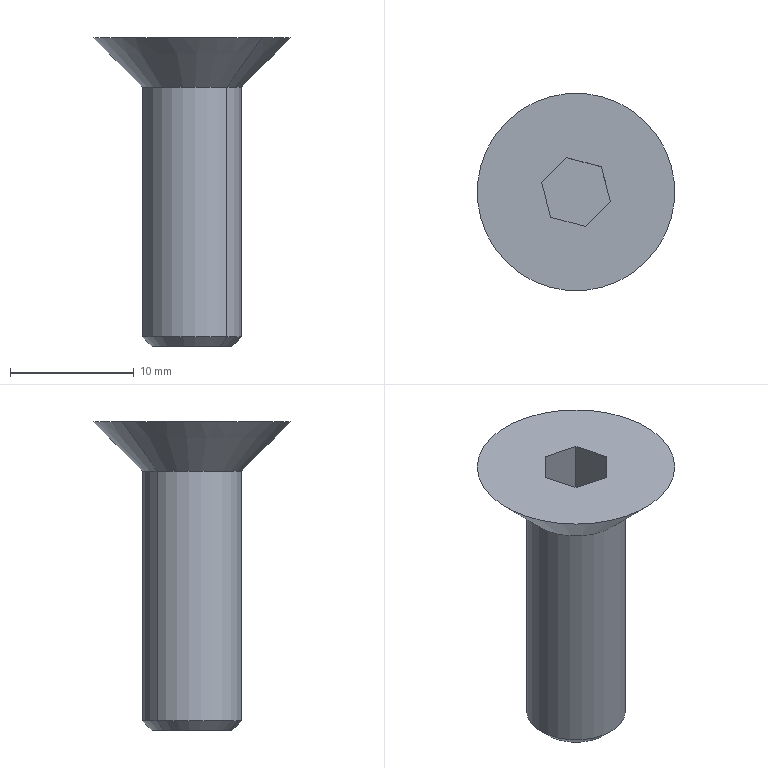Part | NX | features 2 2 | 1 solid | 15 faces | box 16 x 16 x 25 mm | volume 1423 mm3 | plane 9 | cone 4 | cylinder 2 | commonest cylinder face diameters 8 x2
STEP:
#1=CARTESIAN_POINT('',(149.328,-302.828,127.667));
#2=VERTEX_POINT('',#1);
#3=CARTESIAN_POINT('',(148.786,-302.286,126.9));
#4=VERTEX_POINT('',#3);
#5=CARTESIAN_POINT('',(149.057,-302.557,127.284));
#6=DIRECTION('',(-0.5,0.5,-0.7071));
#7=VECTOR('',#6,1000.);
#8=LINE('',#5,#7);
#9=EDGE_CURVE('',#2,#4,#8,.T.);
#10=ORIENTED_EDGE('',*,*,#9,.F.);
#11=CARTESIAN_POINT('',(143.672,-297.172,127.667));
#12=VERTEX_POINT('',#11);
#13=CARTESIAN_POINT('',(146.5,-300.,127.667));
#14=DIRECTION('',(0.,0.,-1.));
#15=DIRECTION('',(0.7071,-0.7071,0.));
#16=AXIS2_PLACEMENT_3D('',#13,#14,#15);
#17=CIRCLE('',#16,4.);
#18=EDGE_CURVE('',#2,#12,#17,.T.);
#19=ORIENTED_EDGE('',*,*,#18,.T.);
#20=CARTESIAN_POINT('',(144.214,-297.714,126.9));
#21=VERTEX_POINT('',#20);
#22=CARTESIAN_POINT('',(143.943,-297.443,127.284));
#23=DIRECTION('',(-0.5,0.5,0.7071));
#24=VECTOR('',#23,1000.);
#25=LINE('',#22,#24);
#26=EDGE_CURVE('',#21,#12,#25,.T.);
#27=ORIENTED_EDGE('',*,*,#26,.F.);
#28=CARTESIAN_POINT('',(146.5,-300.,126.9));
#29=DIRECTION('',(0.,0.,-1.));
#30=DIRECTION('',(0.7071,-0.7071,0.));
#31=AXIS2_PLACEMENT_3D('',#28,#29,#30);
#32=CIRCLE('',#31,3.233);
#33=EDGE_CURVE('',#4,#21,#32,.T.);
#34=ORIENTED_EDGE('',*,*,#33,.F.);
#35=EDGE_LOOP('',(#10,#19,#27,#34));
#36=FACE_BOUND('',#35,.T.);
#37=CARTESIAN_POINT('',(146.5,-300.,127.284));
#38=DIRECTION('',(0.,0.,1.));
#39=DIRECTION('',(0.7071,-0.7071,0.));
#40=AXIS2_PLACEMENT_3D('',#37,#38,#39);
#41=CONICAL_SURFACE('',#40,3.616,0.7854);
#42=ADVANCED_FACE('',(#36),#41,.T.);
#43=CARTESIAN_POINT('',(149.328,-302.828,147.9));
#44=VERTEX_POINT('',#43);
#45=CARTESIAN_POINT('',(149.328,-302.828,137.784));
#46=DIRECTION('',(0.,0.,-1.));
#47=VECTOR('',#46,1000.);
#48=LINE('',#45,#47);
#49=EDGE_CURVE('',#44,#2,#48,.T.);
#50=ORIENTED_EDGE('',*,*,#49,.F.);
#51=CARTESIAN_POINT('',(143.672,-297.172,147.9));
#52=VERTEX_POINT('',#51);
#53=CARTESIAN_POINT('',(146.5,-300.,147.9));
#54=DIRECTION('',(0.,0.,-1.));
#55=DIRECTION('',(0.7071,-0.7071,0.));
#56=AXIS2_PLACEMENT_3D('',#53,#54,#55);
#57=CIRCLE('',#56,4.);
#58=EDGE_CURVE('',#44,#52,#57,.T.);
#59=ORIENTED_EDGE('',*,*,#58,.T.);
#60=CARTESIAN_POINT('',(143.672,-297.172,137.784));
#61=DIRECTION('',(0.,0.,1.));
#62=VECTOR('',#61,1000.);
#63=LINE('',#60,#62);
#64=EDGE_CURVE('',#12,#52,#63,.T.);
#65=ORIENTED_EDGE('',*,*,#64,.F.);
#66=ORIENTED_EDGE('',*,*,#18,.F.);
#67=EDGE_LOOP('',(#50,#59,#65,#66));
#68=FACE_BOUND('',#67,.T.);
#69=CARTESIAN_POINT('',(146.5,-300.,137.784));
#70=DIRECTION('',(0.,0.,1.));
#71=DIRECTION('',(0.7071,-0.7071,0.));
#72=AXIS2_PLACEMENT_3D('',#69,#70,#71);
#73=CYLINDRICAL_SURFACE('',#72,4.);
#74=ADVANCED_FACE('',(#68),#73,.T.);
#75=CARTESIAN_POINT('',(152.157,-305.657,151.9));
#76=VERTEX_POINT('',#75);
#77=CARTESIAN_POINT('',(150.743,-304.243,149.9));
#78=DIRECTION('',(-0.5,0.5,-0.7071));
#79=VECTOR('',#78,1000.);
#80=LINE('',#77,#79);
#81=EDGE_CURVE('',#76,#44,#80,.T.);
#82=ORIENTED_EDGE('',*,*,#81,.F.);
#83=CARTESIAN_POINT('',(140.843,-294.343,151.9));
#84=VERTEX_POINT('',#83);
#85=CARTESIAN_POINT('',(146.5,-300.,151.9));
#86=DIRECTION('',(0.,0.,-1.));
#87=DIRECTION('',(0.7071,-0.7071,0.));
#88=AXIS2_PLACEMENT_3D('',#85,#86,#87);
#89=CIRCLE('',#88,8.);
#90=EDGE_CURVE('',#76,#84,#89,.T.);
#91=ORIENTED_EDGE('',*,*,#90,.T.);
#92=CARTESIAN_POINT('',(142.257,-295.757,149.9));
#93=DIRECTION('',(-0.5,0.5,0.7071));
#94=VECTOR('',#93,1000.);
#95=LINE('',#92,#94);
#96=EDGE_CURVE('',#52,#84,#95,.T.);
#97=ORIENTED_EDGE('',*,*,#96,.F.);
#98=ORIENTED_EDGE('',*,*,#58,.F.);
#99=EDGE_LOOP('',(#82,#91,#97,#98));
#100=FACE_BOUND('',#99,.T.);
#101=CARTESIAN_POINT('',(146.5,-300.,149.9));
#102=DIRECTION('',(0.,0.,1.));
#103=DIRECTION('',(0.7071,-0.7071,0.));
#104=AXIS2_PLACEMENT_3D('',#101,#102,#103);
#105=CONICAL_SURFACE('',#104,6.,0.7854);
#106=ADVANCED_FACE('',(#100),#105,.T.);
#107=CARTESIAN_POINT('',(143.712,-299.253,147.5));
#108=VERTEX_POINT('',#107);
#109=CARTESIAN_POINT('',(144.459,-302.041,147.5));
#110=VERTEX_POINT('',#109);
#111=CARTESIAN_POINT('',(143.712,-299.253,147.5));
#112=DIRECTION('',(0.2588,-0.9659,0.));
#113=VECTOR('',#112,1000.);
#114=LINE('',#111,#113);
#115=EDGE_CURVE('',#108,#110,#114,.T.);
#116=ORIENTED_EDGE('',*,*,#115,.F.);
#117=CARTESIAN_POINT('',(143.712,-299.253,151.9));
#118=VERTEX_POINT('',#117);
#119=CARTESIAN_POINT('',(143.712,-299.253,151.9));
#120=DIRECTION('',(0.,0.,-1.));
#121=VECTOR('',#120,1000.);
#122=LINE('',#119,#121);
#123=EDGE_CURVE('',#118,#108,#122,.T.);
#124=ORIENTED_EDGE('',*,*,#123,.F.);
#125=CARTESIAN_POINT('',(144.459,-302.041,151.9));
#126=VERTEX_POINT('',#125);
#127=CARTESIAN_POINT('',(144.347,-301.623,151.9));
#128=DIRECTION('',(-0.2588,0.9659,0.));
#129=VECTOR('',#128,1000.);
#130=LINE('',#127,#129);
#131=EDGE_CURVE('',#126,#118,#130,.T.);
#132=ORIENTED_EDGE('',*,*,#131,.F.);
#133=CARTESIAN_POINT('',(144.459,-302.041,151.9));
#134=DIRECTION('',(0.,0.,-1.));
#135=VECTOR('',#134,1000.);
#136=LINE('',#133,#135);
#137=EDGE_CURVE('',#126,#110,#136,.T.);
#138=ORIENTED_EDGE('',*,*,#137,.T.);
#139=EDGE_LOOP('',(#116,#124,#132,#138));
#140=FACE_BOUND('',#139,.T.);
#141=CARTESIAN_POINT('',(143.712,-299.253,151.9));
#142=DIRECTION('',(-0.9659,-0.2588,0.));
#143=DIRECTION('',(-0.2588,0.9659,0.));
#144=AXIS2_PLACEMENT_3D('',#141,#142,#143);
#145=PLANE('',#144);
#146=ADVANCED_FACE('',(#140),#145,.F.);
#147=CARTESIAN_POINT('',(147.247,-302.788,147.5));
#148=VERTEX_POINT('',#147);
#149=CARTESIAN_POINT('',(144.459,-302.041,147.5));
#150=DIRECTION('',(0.9659,-0.2588,0.));
#151=VECTOR('',#150,1000.);
#152=LINE('',#149,#151);
#153=EDGE_CURVE('',#110,#148,#152,.T.);
#154=ORIENTED_EDGE('',*,*,#153,.F.);
#155=ORIENTED_EDGE('',*,*,#137,.F.);
#156=CARTESIAN_POINT('',(147.247,-302.788,151.9));
#157=VERTEX_POINT('',#156);
#158=CARTESIAN_POINT('',(146.829,-302.676,151.9));
#159=DIRECTION('',(-0.9659,0.2588,0.));
#160=VECTOR('',#159,1000.);
#161=LINE('',#158,#160);
#162=EDGE_CURVE('',#157,#126,#161,.T.);
#163=ORIENTED_EDGE('',*,*,#162,.F.);
#164=CARTESIAN_POINT('',(147.247,-302.788,151.9));
#165=DIRECTION('',(0.,0.,-1.));
#166=VECTOR('',#165,1000.);
#167=LINE('',#164,#166);
#168=EDGE_CURVE('',#157,#148,#167,.T.);
#169=ORIENTED_EDGE('',*,*,#168,.T.);
#170=EDGE_LOOP('',(#154,#155,#163,#169));
#171=FACE_BOUND('',#170,.T.);
#172=CARTESIAN_POINT('',(144.459,-302.041,151.9));
#173=DIRECTION('',(-0.2588,-0.9659,0.));
#174=DIRECTION('',(-0.9659,0.2588,0.));
#175=AXIS2_PLACEMENT_3D('',#172,#173,#174);
#176=PLANE('',#175);
#177=ADVANCED_FACE('',(#171),#176,.F.);
#178=CARTESIAN_POINT('',(149.288,-300.747,147.5));
#179=VERTEX_POINT('',#178);
#180=CARTESIAN_POINT('',(147.247,-302.788,147.5));
#181=DIRECTION('',(0.7071,0.7071,0.));
#182=VECTOR('',#181,1000.);
#183=LINE('',#180,#182);
#184=EDGE_CURVE('',#148,#179,#183,.T.);
#185=ORIENTED_EDGE('',*,*,#184,.F.);
#186=ORIENTED_EDGE('',*,*,#168,.F.);
#187=CARTESIAN_POINT('',(149.288,-300.747,151.9));
#188=VERTEX_POINT('',#187);
#189=CARTESIAN_POINT('',(147.757,-302.278,151.9));
#190=DIRECTION('',(-0.7071,-0.7071,0.));
#191=VECTOR('',#190,1000.);
#192=LINE('',#189,#191);
#193=EDGE_CURVE('',#188,#157,#192,.T.);
#194=ORIENTED_EDGE('',*,*,#193,.F.);
#195=CARTESIAN_POINT('',(149.288,-300.747,151.9));
#196=DIRECTION('',(0.,0.,-1.));
#197=VECTOR('',#196,1000.);
#198=LINE('',#195,#197);
#199=EDGE_CURVE('',#188,#179,#198,.T.);
#200=ORIENTED_EDGE('',*,*,#199,.T.);
#201=EDGE_LOOP('',(#185,#186,#194,#200));
#202=FACE_BOUND('',#201,.T.);
#203=CARTESIAN_POINT('',(147.247,-302.788,151.9));
#204=DIRECTION('',(0.7071,-0.7071,0.));
#205=DIRECTION('',(-0.7071,-0.7071,0.));
#206=AXIS2_PLACEMENT_3D('',#203,#204,#205);
#207=PLANE('',#206);
#208=ADVANCED_FACE('',(#202),#207,.F.);
#209=CARTESIAN_POINT('',(148.541,-297.959,147.5));
#210=VERTEX_POINT('',#209);
#211=CARTESIAN_POINT('',(149.288,-300.747,147.5));
#212=DIRECTION('',(-0.2588,0.9659,0.));
#213=VECTOR('',#212,1000.);
#214=LINE('',#211,#213);
#215=EDGE_CURVE('',#179,#210,#214,.T.);
#216=ORIENTED_EDGE('',*,*,#215,.F.);
#217=ORIENTED_EDGE('',*,*,#199,.F.);
#218=CARTESIAN_POINT('',(148.541,-297.959,151.9));
#219=VERTEX_POINT('',#218);
#220=CARTESIAN_POINT('',(149.55,-301.723,151.9));
#221=DIRECTION('',(0.2588,-0.9659,0.));
#222=VECTOR('',#221,1000.);
#223=LINE('',#220,#222);
#224=EDGE_CURVE('',#219,#188,#223,.T.);
#225=ORIENTED_EDGE('',*,*,#224,.F.);
#226=CARTESIAN_POINT('',(148.541,-297.959,151.9));
#227=DIRECTION('',(0.,0.,-1.));
#228=VECTOR('',#227,1000.);
#229=LINE('',#226,#228);
#230=EDGE_CURVE('',#219,#210,#229,.T.);
#231=ORIENTED_EDGE('',*,*,#230,.T.);
#232=EDGE_LOOP('',(#216,#217,#225,#231));
#233=FACE_BOUND('',#232,.T.);
#234=CARTESIAN_POINT('',(149.288,-300.747,151.9));
#235=DIRECTION('',(0.9659,0.2588,0.));
#236=DIRECTION('',(0.2588,-0.9659,0.));
#237=AXIS2_PLACEMENT_3D('',#234,#235,#236);
#238=PLANE('',#237);
#239=ADVANCED_FACE('',(#233),#238,.F.);
#240=CARTESIAN_POINT('',(145.753,-297.212,147.5));
#241=VERTEX_POINT('',#240);
#242=CARTESIAN_POINT('',(148.541,-297.959,147.5));
#243=DIRECTION('',(-0.9659,0.2588,0.));
#244=VECTOR('',#243,1000.);
#245=LINE('',#242,#244);
#246=EDGE_CURVE('',#210,#241,#245,.T.);
#247=ORIENTED_EDGE('',*,*,#246,.F.);
#248=ORIENTED_EDGE('',*,*,#230,.F.);
#249=CARTESIAN_POINT('',(145.753,-297.212,151.9));
#250=VERTEX_POINT('',#249);
#251=CARTESIAN_POINT('',(149.517,-298.22,151.9));
#252=DIRECTION('',(0.9659,-0.2588,0.));
#253=VECTOR('',#252,1000.);
#254=LINE('',#251,#253);
#255=EDGE_CURVE('',#250,#219,#254,.T.);
#256=ORIENTED_EDGE('',*,*,#255,.F.);
#257=CARTESIAN_POINT('',(145.753,-297.212,151.9));
#258=DIRECTION('',(0.,0.,-1.));
#259=VECTOR('',#258,1000.);
#260=LINE('',#257,#259);
#261=EDGE_CURVE('',#250,#241,#260,.T.);
#262=ORIENTED_EDGE('',*,*,#261,.T.);
#263=EDGE_LOOP('',(#247,#248,#256,#262));
#264=FACE_BOUND('',#263,.T.);
#265=CARTESIAN_POINT('',(148.541,-297.959,151.9));
#266=DIRECTION('',(0.2588,0.9659,0.));
#267=DIRECTION('',(0.9659,-0.2588,0.));
#268=AXIS2_PLACEMENT_3D('',#265,#266,#267);
#269=PLANE('',#268);
#270=ADVANCED_FACE('',(#264),#269,.F.);
#271=CARTESIAN_POINT('',(145.753,-297.212,147.5));
#272=DIRECTION('',(-0.7071,-0.7071,0.));
#273=VECTOR('',#272,1000.);
#274=LINE('',#271,#273);
#275=EDGE_CURVE('',#241,#108,#274,.T.);
#276=ORIENTED_EDGE('',*,*,#275,.F.);
#277=ORIENTED_EDGE('',*,*,#261,.F.);
#278=CARTESIAN_POINT('',(145.243,-297.722,151.9));
#279=DIRECTION('',(0.7071,0.7071,0.));
#280=VECTOR('',#279,1000.);
#281=LINE('',#278,#280);
#282=EDGE_CURVE('',#118,#250,#281,.T.);
#283=ORIENTED_EDGE('',*,*,#282,.F.);
#284=ORIENTED_EDGE('',*,*,#123,.T.);
#285=EDGE_LOOP('',(#276,#277,#283,#284));
#286=FACE_BOUND('',#285,.T.);
#287=CARTESIAN_POINT('',(145.753,-297.212,151.9));
#288=DIRECTION('',(-0.7071,0.7071,0.));
#289=DIRECTION('',(0.7071,0.7071,0.));
#290=AXIS2_PLACEMENT_3D('',#287,#288,#289);
#291=PLANE('',#290);
#292=ADVANCED_FACE('',(#286),#291,.F.);
#293=ORIENTED_EDGE('',*,*,#115,.T.);
#294=ORIENTED_EDGE('',*,*,#153,.T.);
#295=ORIENTED_EDGE('',*,*,#184,.T.);
#296=ORIENTED_EDGE('',*,*,#215,.T.);
#297=ORIENTED_EDGE('',*,*,#246,.T.);
#298=ORIENTED_EDGE('',*,*,#275,.T.);
#299=EDGE_LOOP('',(#293,#294,#295,#296,#297,#298));
#300=FACE_BOUND('',#299,.T.);
#301=CARTESIAN_POINT('',(146.5,-300.,147.5));
#302=DIRECTION('',(0.,0.,1.));
#303=DIRECTION('',(0.7071,-0.7071,0.));
#304=AXIS2_PLACEMENT_3D('',#301,#302,#303);
#305=PLANE('',#304);
#306=ADVANCED_FACE('',(#300),#305,.T.);
#307=ORIENTED_EDGE('',*,*,#131,.T.);
#308=ORIENTED_EDGE('',*,*,#282,.T.);
#309=ORIENTED_EDGE('',*,*,#255,.T.);
#310=ORIENTED_EDGE('',*,*,#224,.T.);
#311=ORIENTED_EDGE('',*,*,#193,.T.);
#312=ORIENTED_EDGE('',*,*,#162,.T.);
#313=EDGE_LOOP('',(#307,#308,#309,#310,#311,#312));
#314=FACE_BOUND('',#313,.T.);
#315=ORIENTED_EDGE('',*,*,#90,.F.);
#316=CARTESIAN_POINT('',(146.5,-300.,151.9));
#317=DIRECTION('',(0.,0.,-1.));
#318=DIRECTION('',(0.7071,-0.7071,0.));
#319=AXIS2_PLACEMENT_3D('',#316,#317,#318);
#320=CIRCLE('',#319,8.);
#321=EDGE_CURVE('',#84,#76,#320,.T.);
#322=ORIENTED_EDGE('',*,*,#321,.F.);
#323=EDGE_LOOP('',(#315,#322));
#324=FACE_BOUND('',#323,.T.);
#325=CARTESIAN_POINT('',(149.328,-302.828,151.9));
#326=DIRECTION('',(0.,0.,1.));
#327=DIRECTION('',(-0.7071,0.7071,0.));
#328=AXIS2_PLACEMENT_3D('',#325,#326,#327);
#329=PLANE('',#328);
#330=ADVANCED_FACE('',(#314,#324),#329,.T.);
#331=ORIENTED_EDGE('',*,*,#81,.T.);
#332=CARTESIAN_POINT('',(146.5,-300.,147.9));
#333=DIRECTION('',(0.,0.,-1.));
#334=DIRECTION('',(0.7071,-0.7071,0.));
#335=AXIS2_PLACEMENT_3D('',#332,#333,#334);
#336=CIRCLE('',#335,4.);
#337=EDGE_CURVE('',#52,#44,#336,.T.);
#338=ORIENTED_EDGE('',*,*,#337,.F.);
#339=ORIENTED_EDGE('',*,*,#96,.T.);
#340=ORIENTED_EDGE('',*,*,#321,.T.);
#341=EDGE_LOOP('',(#331,#338,#339,#340));
#342=FACE_BOUND('',#341,.T.);
#343=CARTESIAN_POINT('',(146.5,-300.,149.9));
#344=DIRECTION('',(0.,0.,1.));
#345=DIRECTION('',(0.7071,-0.7071,0.));
#346=AXIS2_PLACEMENT_3D('',#343,#344,#345);
#347=CONICAL_SURFACE('',#346,6.,0.7854);
#348=ADVANCED_FACE('',(#342),#347,.T.);
#349=ORIENTED_EDGE('',*,*,#49,.T.);
#350=CARTESIAN_POINT('',(146.5,-300.,127.667));
#351=DIRECTION('',(0.,0.,-1.));
#352=DIRECTION('',(0.7071,-0.7071,0.));
#353=AXIS2_PLACEMENT_3D('',#350,#351,#352);
#354=CIRCLE('',#353,4.);
#355=EDGE_CURVE('',#12,#2,#354,.T.);
#356=ORIENTED_EDGE('',*,*,#355,.F.);
#357=ORIENTED_EDGE('',*,*,#64,.T.);
#358=ORIENTED_EDGE('',*,*,#337,.T.);
#359=EDGE_LOOP('',(#349,#356,#357,#358));
#360=FACE_BOUND('',#359,.T.);
#361=CARTESIAN_POINT('',(146.5,-300.,137.784));
#362=DIRECTION('',(0.,0.,1.));
#363=DIRECTION('',(0.7071,-0.7071,0.));
#364=AXIS2_PLACEMENT_3D('',#361,#362,#363);
#365=CYLINDRICAL_SURFACE('',#364,4.);
#366=ADVANCED_FACE('',(#360),#365,.T.);
#367=ORIENTED_EDGE('',*,*,#9,.T.);
#368=CARTESIAN_POINT('',(146.5,-300.,126.9));
#369=DIRECTION('',(0.,0.,-1.));
#370=DIRECTION('',(0.7071,-0.7071,0.));
#371=AXIS2_PLACEMENT_3D('',#368,#369,#370);
#372=CIRCLE('',#371,3.233);
#373=EDGE_CURVE('',#21,#4,#372,.T.);
#374=ORIENTED_EDGE('',*,*,#373,.F.);
#375=ORIENTED_EDGE('',*,*,#26,.T.);
#376=ORIENTED_EDGE('',*,*,#355,.T.);
#377=EDGE_LOOP('',(#367,#374,#375,#376));
#378=FACE_BOUND('',#377,.T.);
#379=CARTESIAN_POINT('',(146.5,-300.,127.284));
#380=DIRECTION('',(0.,0.,1.));
#381=DIRECTION('',(0.7071,-0.7071,0.));
#382=AXIS2_PLACEMENT_3D('',#379,#380,#381);
#383=CONICAL_SURFACE('',#382,3.616,0.7854);
#384=ADVANCED_FACE('',(#378),#383,.T.);
#385=ORIENTED_EDGE('',*,*,#33,.T.);
#386=ORIENTED_EDGE('',*,*,#373,.T.);
#387=EDGE_LOOP('',(#385,#386));
#388=FACE_BOUND('',#387,.T.);
#389=CARTESIAN_POINT('',(147.643,-301.143,126.9));
#390=DIRECTION('',(0.,0.,-1.));
#391=DIRECTION('',(0.7071,-0.7071,0.));
#392=AXIS2_PLACEMENT_3D('',#389,#390,#391);
#393=PLANE('',#392);
#394=ADVANCED_FACE('',(#388),#393,.T.);
#395=CLOSED_SHELL('',(#42,#74,#106,#146,#177,#208,#239,#270,#292,#306,#330,#348,#366,#384,#394));
#396=MANIFOLD_SOLID_BREP('',#395);
#397=(LENGTH_UNIT()NAMED_UNIT(*)SI_UNIT(.MILLI.,.METRE.));
#398=UNCERTAINTY_MEASURE_WITH_UNIT(LENGTH_MEASURE(0.00001),#397,'','');
#399=(NAMED_UNIT(*)PLANE_ANGLE_UNIT()SI_UNIT($,.RADIAN.));
#400=(NAMED_UNIT(*)SI_UNIT($,.STERADIAN.)SOLID_ANGLE_UNIT());
#401=(GEOMETRIC_REPRESENTATION_CONTEXT(3)GLOBAL_UNCERTAINTY_ASSIGNED_CONTEXT((#398))GLOBAL_UNIT_ASSIGNED_CONTEXT((#397,#399,#400))REPRESENTATION_CONTEXT('',''));
#402=ADVANCED_BREP_SHAPE_REPRESENTATION('',(#396),#401);